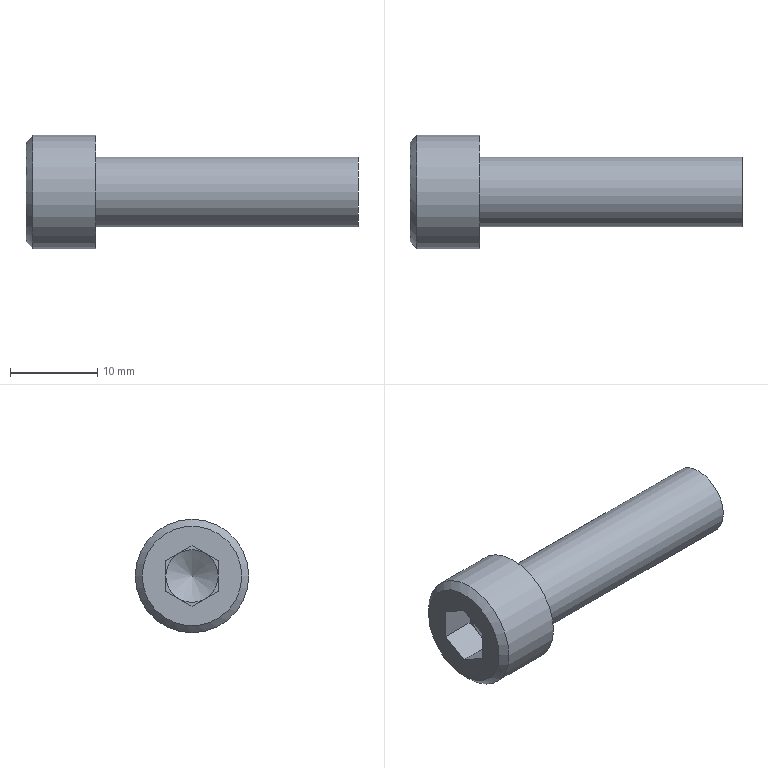Part | NX | features 5003_324_CB8-30 2 | 1 solid | 19 faces | box 38 x 13 x 13 mm | volume 2416 mm3 | plane 15 | cylinder 2 | cone 2 | commonest cylinder face diameters 8 x1 13 x1
STEP:
#1=CARTESIAN_POINT('',(375.29,-28.2,-129.25));
#2=VERTEX_POINT('',#1);
#3=CARTESIAN_POINT('',(375.29,-22.5,-129.25));
#4=DIRECTION('',(1.,0.,0.));
#5=DIRECTION('',(0.,-1.,0.));
#6=AXIS2_PLACEMENT_3D('',#3,#4,#5);
#7=CIRCLE('',#6,5.7);
#8=EDGE_CURVE('',#2,#2,#7,.F.);
#9=ORIENTED_EDGE('',*,*,#8,.T.);
#10=EDGE_LOOP('',(#9));
#11=FACE_BOUND('',#10,.T.);
#12=CARTESIAN_POINT('',(375.29,-22.5,-125.786));
#13=VERTEX_POINT('',#12);
#14=CARTESIAN_POINT('',(375.29,-19.5,-127.518));
#15=VERTEX_POINT('',#14);
#16=CARTESIAN_POINT('',(375.29,-22.5,-125.786));
#17=DIRECTION('',(0.,0.866,-0.5));
#18=VECTOR('',#17,1000.);
#19=LINE('',#16,#18);
#20=EDGE_CURVE('',#13,#15,#19,.T.);
#21=ORIENTED_EDGE('',*,*,#20,.F.);
#22=CARTESIAN_POINT('',(375.29,-25.5,-127.518));
#23=VERTEX_POINT('',#22);
#24=CARTESIAN_POINT('',(375.29,-25.5,-127.518));
#25=DIRECTION('',(0.,0.866,0.5));
#26=VECTOR('',#25,1000.);
#27=LINE('',#24,#26);
#28=EDGE_CURVE('',#23,#13,#27,.T.);
#29=ORIENTED_EDGE('',*,*,#28,.F.);
#30=CARTESIAN_POINT('',(375.29,-25.5,-130.982));
#31=VERTEX_POINT('',#30);
#32=CARTESIAN_POINT('',(375.29,-25.5,-130.982));
#33=DIRECTION('',(0.,0.,1.));
#34=VECTOR('',#33,1000.);
#35=LINE('',#32,#34);
#36=EDGE_CURVE('',#31,#23,#35,.T.);
#37=ORIENTED_EDGE('',*,*,#36,.F.);
#38=CARTESIAN_POINT('',(375.29,-22.5,-132.714));
#39=VERTEX_POINT('',#38);
#40=CARTESIAN_POINT('',(375.29,-22.5,-132.714));
#41=DIRECTION('',(0.,-0.866,0.5));
#42=VECTOR('',#41,1000.);
#43=LINE('',#40,#42);
#44=EDGE_CURVE('',#39,#31,#43,.T.);
#45=ORIENTED_EDGE('',*,*,#44,.F.);
#46=CARTESIAN_POINT('',(375.29,-19.5,-130.982));
#47=VERTEX_POINT('',#46);
#48=CARTESIAN_POINT('',(375.29,-19.5,-130.982));
#49=DIRECTION('',(0.,-0.866,-0.5));
#50=VECTOR('',#49,1000.);
#51=LINE('',#48,#50);
#52=EDGE_CURVE('',#47,#39,#51,.T.);
#53=ORIENTED_EDGE('',*,*,#52,.F.);
#54=CARTESIAN_POINT('',(375.29,-19.5,-127.518));
#55=DIRECTION('',(0.,0.,-1.));
#56=VECTOR('',#55,1000.);
#57=LINE('',#54,#56);
#58=EDGE_CURVE('',#15,#47,#57,.T.);
#59=ORIENTED_EDGE('',*,*,#58,.F.);
#60=EDGE_LOOP('',(#21,#29,#37,#45,#53,#59));
#61=FACE_BOUND('',#60,.T.);
#62=CARTESIAN_POINT('',(375.29,-22.5,-135.75));
#63=DIRECTION('',(1.,0.,0.));
#64=DIRECTION('',(0.,-1.,0.));
#65=AXIS2_PLACEMENT_3D('',#62,#63,#64);
#66=PLANE('',#65);
#67=ADVANCED_FACE('',(#11,#61),#66,.F.);
#68=CARTESIAN_POINT('',(413.29,-18.5,-129.25));
#69=VERTEX_POINT('',#68);
#70=CARTESIAN_POINT('',(413.29,-22.5,-129.25));
#71=DIRECTION('',(-1.,0.,0.));
#72=DIRECTION('',(0.,1.,0.));
#73=AXIS2_PLACEMENT_3D('',#70,#71,#72);
#74=CIRCLE('',#73,4.);
#75=EDGE_CURVE('',#69,#69,#74,.T.);
#76=ORIENTED_EDGE('',*,*,#75,.F.);
#77=EDGE_LOOP('',(#76));
#78=FACE_BOUND('',#77,.T.);
#79=CARTESIAN_POINT('',(413.29,-22.5,-129.25));
#80=DIRECTION('',(-1.,0.,0.));
#81=DIRECTION('',(0.,1.,0.));
#82=AXIS2_PLACEMENT_3D('',#79,#80,#81);
#83=PLANE('',#82);
#84=ADVANCED_FACE('',(#78),#83,.F.);
#85=CARTESIAN_POINT('',(383.29,-18.5,-129.25));
#86=VERTEX_POINT('',#85);
#87=CARTESIAN_POINT('',(383.29,-22.5,-129.25));
#88=DIRECTION('',(-1.,0.,0.));
#89=DIRECTION('',(0.,1.,0.));
#90=AXIS2_PLACEMENT_3D('',#87,#88,#89);
#91=CIRCLE('',#90,4.);
#92=EDGE_CURVE('',#86,#86,#91,.T.);
#93=ORIENTED_EDGE('',*,*,#92,.F.);
#94=EDGE_LOOP('',(#93));
#95=FACE_BOUND('',#94,.T.);
#96=ORIENTED_EDGE('',*,*,#75,.T.);
#97=EDGE_LOOP('',(#96));
#98=FACE_BOUND('',#97,.T.);
#99=CARTESIAN_POINT('',(375.29,-22.5,-129.25));
#100=DIRECTION('',(-1.,0.,0.));
#101=DIRECTION('',(0.,1.,0.));
#102=AXIS2_PLACEMENT_3D('',#99,#100,#101);
#103=CYLINDRICAL_SURFACE('',#102,4.);
#104=ADVANCED_FACE('',(#95,#98),#103,.T.);
#105=CARTESIAN_POINT('',(383.29,-16.,-129.25));
#106=VERTEX_POINT('',#105);
#107=CARTESIAN_POINT('',(383.29,-22.5,-129.25));
#108=DIRECTION('',(-1.,0.,0.));
#109=DIRECTION('',(0.,1.,0.));
#110=AXIS2_PLACEMENT_3D('',#107,#108,#109);
#111=CIRCLE('',#110,6.5);
#112=EDGE_CURVE('',#106,#106,#111,.T.);
#113=ORIENTED_EDGE('',*,*,#112,.F.);
#114=EDGE_LOOP('',(#113));
#115=FACE_BOUND('',#114,.T.);
#116=ORIENTED_EDGE('',*,*,#92,.T.);
#117=EDGE_LOOP('',(#116));
#118=FACE_BOUND('',#117,.T.);
#119=CARTESIAN_POINT('',(383.29,-22.5,-133.25));
#120=DIRECTION('',(-1.,0.,0.));
#121=DIRECTION('',(0.,1.,0.));
#122=AXIS2_PLACEMENT_3D('',#119,#120,#121);
#123=PLANE('',#122);
#124=ADVANCED_FACE('',(#115,#118),#123,.F.);
#125=CARTESIAN_POINT('',(376.09,-29.,-129.25));
#126=VERTEX_POINT('',#125);
#127=CARTESIAN_POINT('',(376.09,-22.5,-129.25));
#128=DIRECTION('',(1.,0.,0.));
#129=DIRECTION('',(0.,-1.,0.));
#130=AXIS2_PLACEMENT_3D('',#127,#128,#129);
#131=CIRCLE('',#130,6.5);
#132=EDGE_CURVE('',#126,#126,#131,.T.);
#133=ORIENTED_EDGE('',*,*,#132,.T.);
#134=EDGE_LOOP('',(#133));
#135=FACE_BOUND('',#134,.T.);
#136=ORIENTED_EDGE('',*,*,#112,.T.);
#137=EDGE_LOOP('',(#136));
#138=FACE_BOUND('',#137,.T.);
#139=CARTESIAN_POINT('',(375.29,-22.5,-129.25));
#140=DIRECTION('',(-1.,0.,0.));
#141=DIRECTION('',(0.,1.,0.));
#142=AXIS2_PLACEMENT_3D('',#139,#140,#141);
#143=CYLINDRICAL_SURFACE('',#142,6.5);
#144=ADVANCED_FACE('',(#135,#138),#143,.T.);
#145=ORIENTED_EDGE('',*,*,#132,.F.);
#146=EDGE_LOOP('',(#145));
#147=FACE_BOUND('',#146,.T.);
#148=ORIENTED_EDGE('',*,*,#8,.F.);
#149=EDGE_LOOP('',(#148));
#150=FACE_BOUND('',#149,.T.);
#151=CARTESIAN_POINT('',(375.29,-22.5,-129.25));
#152=DIRECTION('',(1.,0.,0.));
#153=DIRECTION('',(0.,-1.,0.));
#154=AXIS2_PLACEMENT_3D('',#151,#152,#153);
#155=CONICAL_SURFACE('',#154,5.7,0.7854);
#156=ADVANCED_FACE('',(#147,#150),#155,.T.);
#157=CARTESIAN_POINT('',(379.29,-25.5,-127.518));
#158=VERTEX_POINT('',#157);
#159=CARTESIAN_POINT('',(379.29,-24.,-126.652));
#160=VERTEX_POINT('',#159);
#161=CARTESIAN_POINT('',(379.29,-25.5,-127.518));
#162=DIRECTION('',(0.,0.866,0.5));
#163=VECTOR('',#162,1000.);
#164=LINE('',#161,#163);
#165=EDGE_CURVE('',#158,#160,#164,.T.);
#166=ORIENTED_EDGE('',*,*,#165,.F.);
#167=CARTESIAN_POINT('',(379.29,-25.5,-127.518));
#168=DIRECTION('',(-1.,0.,0.));
#169=VECTOR('',#168,1000.);
#170=LINE('',#167,#169);
#171=EDGE_CURVE('',#158,#23,#170,.T.);
#172=ORIENTED_EDGE('',*,*,#171,.T.);
#173=ORIENTED_EDGE('',*,*,#28,.T.);
#174=CARTESIAN_POINT('',(379.29,-22.5,-125.786));
#175=VERTEX_POINT('',#174);
#176=CARTESIAN_POINT('',(379.29,-22.5,-125.786));
#177=DIRECTION('',(-1.,0.,0.));
#178=VECTOR('',#177,1000.);
#179=LINE('',#176,#178);
#180=EDGE_CURVE('',#175,#13,#179,.T.);
#181=ORIENTED_EDGE('',*,*,#180,.F.);
#182=CARTESIAN_POINT('',(379.29,-25.5,-127.518));
#183=DIRECTION('',(0.,0.866,0.5));
#184=VECTOR('',#183,1000.);
#185=LINE('',#182,#184);
#186=EDGE_CURVE('',#160,#175,#185,.T.);
#187=ORIENTED_EDGE('',*,*,#186,.F.);
#188=EDGE_LOOP('',(#166,#172,#173,#181,#187));
#189=FACE_BOUND('',#188,.T.);
#190=CARTESIAN_POINT('',(379.29,-25.5,-127.518));
#191=DIRECTION('',(0.,-0.5,0.866));
#192=DIRECTION('',(0.,-0.866,-0.5));
#193=AXIS2_PLACEMENT_3D('',#190,#191,#192);
#194=PLANE('',#193);
#195=ADVANCED_FACE('',(#189),#194,.F.);
#196=CARTESIAN_POINT('',(379.29,-25.5,-130.982));
#197=VERTEX_POINT('',#196);
#198=CARTESIAN_POINT('',(379.29,-25.5,-129.25));
#199=VERTEX_POINT('',#198);
#200=CARTESIAN_POINT('',(379.29,-25.5,-130.982));
#201=DIRECTION('',(0.,0.,1.));
#202=VECTOR('',#201,1000.);
#203=LINE('',#200,#202);
#204=EDGE_CURVE('',#197,#199,#203,.T.);
#205=ORIENTED_EDGE('',*,*,#204,.F.);
#206=CARTESIAN_POINT('',(379.29,-25.5,-130.982));
#207=DIRECTION('',(-1.,0.,0.));
#208=VECTOR('',#207,1000.);
#209=LINE('',#206,#208);
#210=EDGE_CURVE('',#197,#31,#209,.T.);
#211=ORIENTED_EDGE('',*,*,#210,.T.);
#212=ORIENTED_EDGE('',*,*,#36,.T.);
#213=ORIENTED_EDGE('',*,*,#171,.F.);
#214=CARTESIAN_POINT('',(379.29,-25.5,-130.982));
#215=DIRECTION('',(0.,0.,1.));
#216=VECTOR('',#215,1000.);
#217=LINE('',#214,#216);
#218=EDGE_CURVE('',#199,#158,#217,.T.);
#219=ORIENTED_EDGE('',*,*,#218,.F.);
#220=EDGE_LOOP('',(#205,#211,#212,#213,#219));
#221=FACE_BOUND('',#220,.T.);
#222=CARTESIAN_POINT('',(379.29,-25.5,-130.982));
#223=DIRECTION('',(0.,-1.,0.));
#224=DIRECTION('',(-1.,0.,0.));
#225=AXIS2_PLACEMENT_3D('',#222,#223,#224);
#226=PLANE('',#225);
#227=ADVANCED_FACE('',(#221),#226,.F.);
#228=CARTESIAN_POINT('',(379.29,-22.5,-132.714));
#229=VERTEX_POINT('',#228);
#230=CARTESIAN_POINT('',(379.29,-24.,-131.848));
#231=VERTEX_POINT('',#230);
#232=CARTESIAN_POINT('',(379.29,-22.5,-132.714));
#233=DIRECTION('',(0.,-0.866,0.5));
#234=VECTOR('',#233,1000.);
#235=LINE('',#232,#234);
#236=EDGE_CURVE('',#229,#231,#235,.T.);
#237=ORIENTED_EDGE('',*,*,#236,.F.);
#238=CARTESIAN_POINT('',(379.29,-22.5,-132.714));
#239=DIRECTION('',(-1.,0.,0.));
#240=VECTOR('',#239,1000.);
#241=LINE('',#238,#240);
#242=EDGE_CURVE('',#229,#39,#241,.T.);
#243=ORIENTED_EDGE('',*,*,#242,.T.);
#244=ORIENTED_EDGE('',*,*,#44,.T.);
#245=ORIENTED_EDGE('',*,*,#210,.F.);
#246=CARTESIAN_POINT('',(379.29,-22.5,-132.714));
#247=DIRECTION('',(0.,-0.866,0.5));
#248=VECTOR('',#247,1000.);
#249=LINE('',#246,#248);
#250=EDGE_CURVE('',#231,#197,#249,.T.);
#251=ORIENTED_EDGE('',*,*,#250,.F.);
#252=EDGE_LOOP('',(#237,#243,#244,#245,#251));
#253=FACE_BOUND('',#252,.T.);
#254=CARTESIAN_POINT('',(379.29,-22.5,-132.714));
#255=DIRECTION('',(0.,-0.5,-0.866));
#256=DIRECTION('',(0.,0.866,-0.5));
#257=AXIS2_PLACEMENT_3D('',#254,#255,#256);
#258=PLANE('',#257);
#259=ADVANCED_FACE('',(#253),#258,.F.);
#260=CARTESIAN_POINT('',(379.29,-19.5,-130.982));
#261=VERTEX_POINT('',#260);
#262=CARTESIAN_POINT('',(379.29,-21.,-131.848));
#263=VERTEX_POINT('',#262);
#264=CARTESIAN_POINT('',(379.29,-19.5,-130.982));
#265=DIRECTION('',(0.,-0.866,-0.5));
#266=VECTOR('',#265,1000.);
#267=LINE('',#264,#266);
#268=EDGE_CURVE('',#261,#263,#267,.T.);
#269=ORIENTED_EDGE('',*,*,#268,.F.);
#270=CARTESIAN_POINT('',(379.29,-19.5,-130.982));
#271=DIRECTION('',(-1.,0.,0.));
#272=VECTOR('',#271,1000.);
#273=LINE('',#270,#272);
#274=EDGE_CURVE('',#261,#47,#273,.T.);
#275=ORIENTED_EDGE('',*,*,#274,.T.);
#276=ORIENTED_EDGE('',*,*,#52,.T.);
#277=ORIENTED_EDGE('',*,*,#242,.F.);
#278=CARTESIAN_POINT('',(379.29,-19.5,-130.982));
#279=DIRECTION('',(0.,-0.866,-0.5));
#280=VECTOR('',#279,1000.);
#281=LINE('',#278,#280);
#282=EDGE_CURVE('',#263,#229,#281,.T.);
#283=ORIENTED_EDGE('',*,*,#282,.F.);
#284=EDGE_LOOP('',(#269,#275,#276,#277,#283));
#285=FACE_BOUND('',#284,.T.);
#286=CARTESIAN_POINT('',(379.29,-19.5,-130.982));
#287=DIRECTION('',(0.,0.5,-0.866));
#288=DIRECTION('',(0.,0.866,0.5));
#289=AXIS2_PLACEMENT_3D('',#286,#287,#288);
#290=PLANE('',#289);
#291=ADVANCED_FACE('',(#285),#290,.F.);
#292=CARTESIAN_POINT('',(379.29,-19.5,-127.518));
#293=VERTEX_POINT('',#292);
#294=CARTESIAN_POINT('',(379.29,-19.5,-129.25));
#295=VERTEX_POINT('',#294);
#296=CARTESIAN_POINT('',(379.29,-19.5,-127.518));
#297=DIRECTION('',(0.,0.,-1.));
#298=VECTOR('',#297,1000.);
#299=LINE('',#296,#298);
#300=EDGE_CURVE('',#293,#295,#299,.T.);
#301=ORIENTED_EDGE('',*,*,#300,.F.);
#302=CARTESIAN_POINT('',(379.29,-19.5,-127.518));
#303=DIRECTION('',(-1.,0.,0.));
#304=VECTOR('',#303,1000.);
#305=LINE('',#302,#304);
#306=EDGE_CURVE('',#293,#15,#305,.T.);
#307=ORIENTED_EDGE('',*,*,#306,.T.);
#308=ORIENTED_EDGE('',*,*,#58,.T.);
#309=ORIENTED_EDGE('',*,*,#274,.F.);
#310=CARTESIAN_POINT('',(379.29,-19.5,-127.518));
#311=DIRECTION('',(0.,0.,-1.));
#312=VECTOR('',#311,1000.);
#313=LINE('',#310,#312);
#314=EDGE_CURVE('',#295,#261,#313,.T.);
#315=ORIENTED_EDGE('',*,*,#314,.F.);
#316=EDGE_LOOP('',(#301,#307,#308,#309,#315));
#317=FACE_BOUND('',#316,.T.);
#318=CARTESIAN_POINT('',(379.29,-19.5,-127.518));
#319=DIRECTION('',(0.,1.,0.));
#320=DIRECTION('',(0.,0.,1.));
#321=AXIS2_PLACEMENT_3D('',#318,#319,#320);
#322=PLANE('',#321);
#323=ADVANCED_FACE('',(#317),#322,.F.);
#324=CARTESIAN_POINT('',(379.29,-21.,-126.652));
#325=VERTEX_POINT('',#324);
#326=CARTESIAN_POINT('',(379.29,-22.5,-125.786));
#327=DIRECTION('',(0.,0.866,-0.5));
#328=VECTOR('',#327,1000.);
#329=LINE('',#326,#328);
#330=EDGE_CURVE('',#175,#325,#329,.T.);
#331=ORIENTED_EDGE('',*,*,#330,.F.);
#332=ORIENTED_EDGE('',*,*,#180,.T.);
#333=ORIENTED_EDGE('',*,*,#20,.T.);
#334=ORIENTED_EDGE('',*,*,#306,.F.);
#335=CARTESIAN_POINT('',(379.29,-22.5,-125.786));
#336=DIRECTION('',(0.,0.866,-0.5));
#337=VECTOR('',#336,1000.);
#338=LINE('',#335,#337);
#339=EDGE_CURVE('',#325,#293,#338,.T.);
#340=ORIENTED_EDGE('',*,*,#339,.F.);
#341=EDGE_LOOP('',(#331,#332,#333,#334,#340));
#342=FACE_BOUND('',#341,.T.);
#343=CARTESIAN_POINT('',(379.29,-22.5,-125.786));
#344=DIRECTION('',(0.,0.5,0.866));
#345=DIRECTION('',(0.,-0.866,0.5));
#346=AXIS2_PLACEMENT_3D('',#343,#344,#345);
#347=PLANE('',#346);
#348=ADVANCED_FACE('',(#342),#347,.F.);
#349=ORIENTED_EDGE('',*,*,#314,.T.);
#350=ORIENTED_EDGE('',*,*,#268,.T.);
#351=CARTESIAN_POINT('',(379.29,-22.5,-129.25));
#352=DIRECTION('',(-1.,0.,0.));
#353=DIRECTION('',(0.,0.,1.));
#354=AXIS2_PLACEMENT_3D('',#351,#352,#353);
#355=CIRCLE('',#354,3.);
#356=EDGE_CURVE('',#295,#263,#355,.T.);
#357=ORIENTED_EDGE('',*,*,#356,.F.);
#358=EDGE_LOOP('',(#349,#350,#357));
#359=FACE_BOUND('',#358,.T.);
#360=CARTESIAN_POINT('',(379.29,-22.5,-129.25));
#361=DIRECTION('',(-1.,0.,0.));
#362=DIRECTION('',(0.,1.,0.));
#363=AXIS2_PLACEMENT_3D('',#360,#361,#362);
#364=PLANE('',#363);
#365=ADVANCED_FACE('',(#359),#364,.T.);
#366=ORIENTED_EDGE('',*,*,#282,.T.);
#367=ORIENTED_EDGE('',*,*,#236,.T.);
#368=CARTESIAN_POINT('',(379.29,-22.5,-129.25));
#369=DIRECTION('',(-1.,0.,0.));
#370=DIRECTION('',(0.,0.,1.));
#371=AXIS2_PLACEMENT_3D('',#368,#369,#370);
#372=CIRCLE('',#371,3.);
#373=EDGE_CURVE('',#263,#231,#372,.T.);
#374=ORIENTED_EDGE('',*,*,#373,.F.);
#375=EDGE_LOOP('',(#366,#367,#374));
#376=FACE_BOUND('',#375,.T.);
#377=CARTESIAN_POINT('',(379.29,-22.5,-129.25));
#378=DIRECTION('',(-1.,0.,0.));
#379=DIRECTION('',(0.,1.,0.));
#380=AXIS2_PLACEMENT_3D('',#377,#378,#379);
#381=PLANE('',#380);
#382=ADVANCED_FACE('',(#376),#381,.T.);
#383=ORIENTED_EDGE('',*,*,#250,.T.);
#384=ORIENTED_EDGE('',*,*,#204,.T.);
#385=CARTESIAN_POINT('',(379.29,-22.5,-129.25));
#386=DIRECTION('',(-1.,0.,0.));
#387=DIRECTION('',(0.,0.,1.));
#388=AXIS2_PLACEMENT_3D('',#385,#386,#387);
#389=CIRCLE('',#388,3.);
#390=EDGE_CURVE('',#231,#199,#389,.T.);
#391=ORIENTED_EDGE('',*,*,#390,.F.);
#392=EDGE_LOOP('',(#383,#384,#391));
#393=FACE_BOUND('',#392,.T.);
#394=CARTESIAN_POINT('',(379.29,-22.5,-129.25));
#395=DIRECTION('',(-1.,0.,0.));
#396=DIRECTION('',(0.,1.,0.));
#397=AXIS2_PLACEMENT_3D('',#394,#395,#396);
#398=PLANE('',#397);
#399=ADVANCED_FACE('',(#393),#398,.T.);
#400=ORIENTED_EDGE('',*,*,#218,.T.);
#401=ORIENTED_EDGE('',*,*,#165,.T.);
#402=CARTESIAN_POINT('',(379.29,-22.5,-129.25));
#403=DIRECTION('',(-1.,0.,0.));
#404=DIRECTION('',(0.,0.,1.));
#405=AXIS2_PLACEMENT_3D('',#402,#403,#404);
#406=CIRCLE('',#405,3.);
#407=EDGE_CURVE('',#199,#160,#406,.T.);
#408=ORIENTED_EDGE('',*,*,#407,.F.);
#409=EDGE_LOOP('',(#400,#401,#408));
#410=FACE_BOUND('',#409,.T.);
#411=CARTESIAN_POINT('',(379.29,-22.5,-129.25));
#412=DIRECTION('',(-1.,0.,0.));
#413=DIRECTION('',(0.,1.,0.));
#414=AXIS2_PLACEMENT_3D('',#411,#412,#413);
#415=PLANE('',#414);
#416=ADVANCED_FACE('',(#410),#415,.T.);
#417=ORIENTED_EDGE('',*,*,#186,.T.);
#418=ORIENTED_EDGE('',*,*,#330,.T.);
#419=CARTESIAN_POINT('',(379.29,-22.5,-129.25));
#420=DIRECTION('',(-1.,0.,0.));
#421=DIRECTION('',(0.,0.,1.));
#422=AXIS2_PLACEMENT_3D('',#419,#420,#421);
#423=CIRCLE('',#422,3.);
#424=EDGE_CURVE('',#160,#325,#423,.T.);
#425=ORIENTED_EDGE('',*,*,#424,.F.);
#426=EDGE_LOOP('',(#417,#418,#425));
#427=FACE_BOUND('',#426,.T.);
#428=CARTESIAN_POINT('',(379.29,-22.5,-129.25));
#429=DIRECTION('',(-1.,0.,0.));
#430=DIRECTION('',(0.,1.,0.));
#431=AXIS2_PLACEMENT_3D('',#428,#429,#430);
#432=PLANE('',#431);
#433=ADVANCED_FACE('',(#427),#432,.T.);
#434=ORIENTED_EDGE('',*,*,#339,.T.);
#435=ORIENTED_EDGE('',*,*,#300,.T.);
#436=CARTESIAN_POINT('',(379.29,-22.5,-129.25));
#437=DIRECTION('',(-1.,0.,0.));
#438=DIRECTION('',(0.,0.,1.));
#439=AXIS2_PLACEMENT_3D('',#436,#437,#438);
#440=CIRCLE('',#439,3.);
#441=EDGE_CURVE('',#325,#295,#440,.T.);
#442=ORIENTED_EDGE('',*,*,#441,.F.);
#443=EDGE_LOOP('',(#434,#435,#442));
#444=FACE_BOUND('',#443,.T.);
#445=CARTESIAN_POINT('',(379.29,-22.5,-129.25));
#446=DIRECTION('',(-1.,0.,0.));
#447=DIRECTION('',(0.,1.,0.));
#448=AXIS2_PLACEMENT_3D('',#445,#446,#447);
#449=PLANE('',#448);
#450=ADVANCED_FACE('',(#444),#449,.T.);
#451=ORIENTED_EDGE('',*,*,#441,.T.);
#452=ORIENTED_EDGE('',*,*,#356,.T.);
#453=ORIENTED_EDGE('',*,*,#373,.T.);
#454=ORIENTED_EDGE('',*,*,#390,.T.);
#455=ORIENTED_EDGE('',*,*,#407,.T.);
#456=ORIENTED_EDGE('',*,*,#424,.T.);
#457=EDGE_LOOP('',(#451,#452,#453,#454,#455,#456));
#458=FACE_BOUND('',#457,.T.);
#459=CARTESIAN_POINT('',(381.093,-22.5,-129.25));
#460=VERTEX_POINT('',#459);
#461=VERTEX_LOOP('',#460);
#462=FACE_BOUND('',#461,.T.);
#463=CARTESIAN_POINT('',(381.093,-22.5,-129.25));
#464=DIRECTION('',(-1.,0.,0.));
#465=DIRECTION('',(0.,0.,1.));
#466=AXIS2_PLACEMENT_3D('',#463,#464,#465);
#467=CONICAL_SURFACE('',#466,0.,1.03);
#468=ADVANCED_FACE('',(#458,#462),#467,.F.);
#469=CLOSED_SHELL('',(#67,#84,#104,#124,#144,#156,#195,#227,#259,#291,#323,#348,#365,#382,#399,#416,#433,#450,#468));
#470=MANIFOLD_SOLID_BREP('',#469);
#471=(LENGTH_UNIT()NAMED_UNIT(*)SI_UNIT(.MILLI.,.METRE.));
#472=UNCERTAINTY_MEASURE_WITH_UNIT(LENGTH_MEASURE(0.00001),#471,'','');
#473=(NAMED_UNIT(*)PLANE_ANGLE_UNIT()SI_UNIT($,.RADIAN.));
#474=(NAMED_UNIT(*)SI_UNIT($,.STERADIAN.)SOLID_ANGLE_UNIT());
#475=(GEOMETRIC_REPRESENTATION_CONTEXT(3)GLOBAL_UNCERTAINTY_ASSIGNED_CONTEXT((#472))GLOBAL_UNIT_ASSIGNED_CONTEXT((#471,#473,#474))REPRESENTATION_CONTEXT('',''));
#476=ADVANCED_BREP_SHAPE_REPRESENTATION('',(#470),#475);